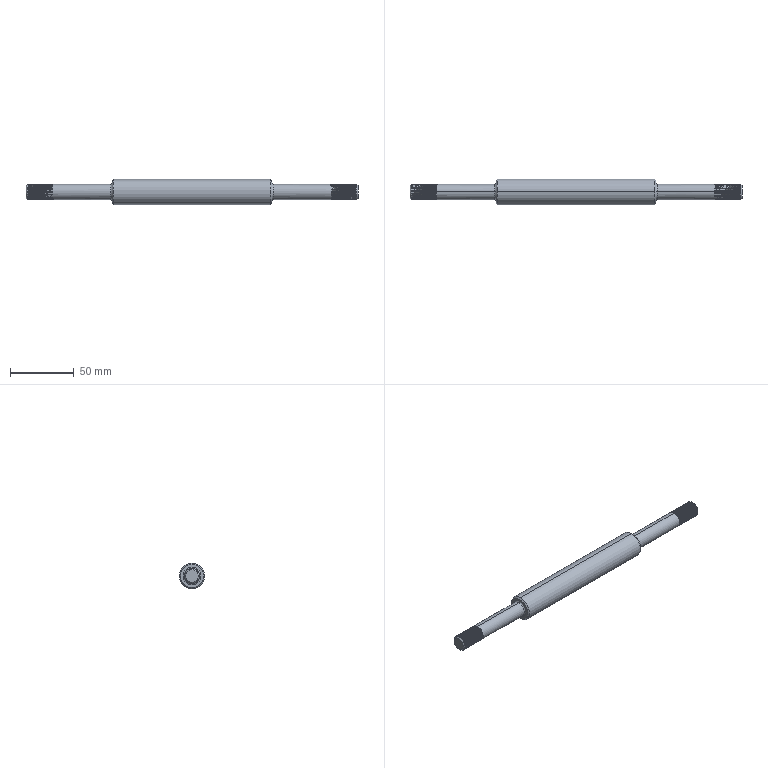Part | STEP file | Hinge pin stepped shaft | 1 solid | 232 faces | box 260 x 20 x 20 mm | volume 54217 mm3 | cylinder 206 | cone 8 | plane 8 | spline 6 | torus 4 | commonest cylinder face diameters 12 x204 20 x2